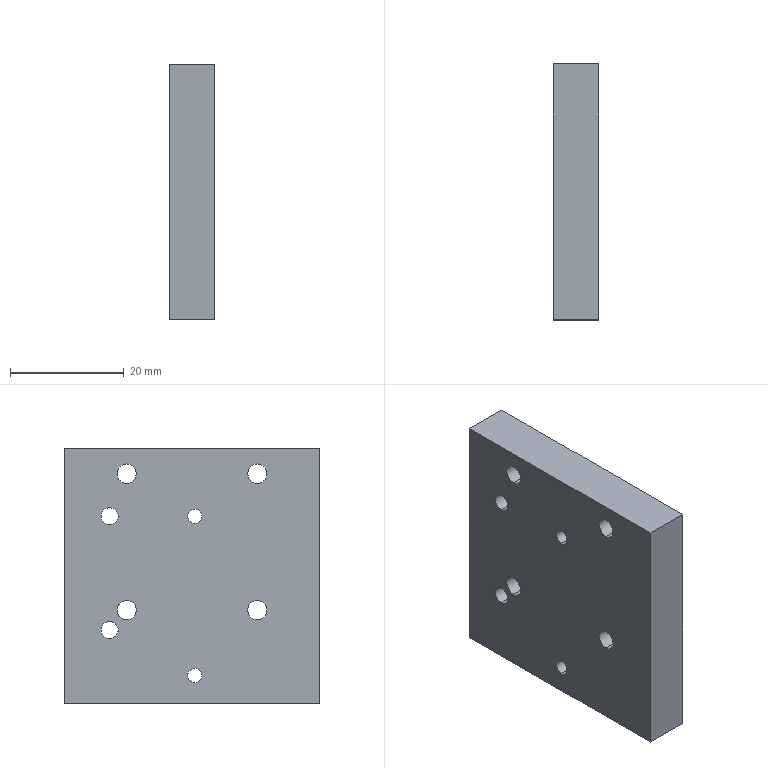Part | SolidWorks | features LPattern 5, HoleWzd 4, Extrusion 1 | 1 solid | 46 faces | box 8 x 45 x 45 mm | volume 15170 mm3 | cylinder 31 | plane 10 | cone 5 | commonest cylinder face diameters 6.5 x9 3.4 x8 3.3 x6 2.5 x4 3 x4